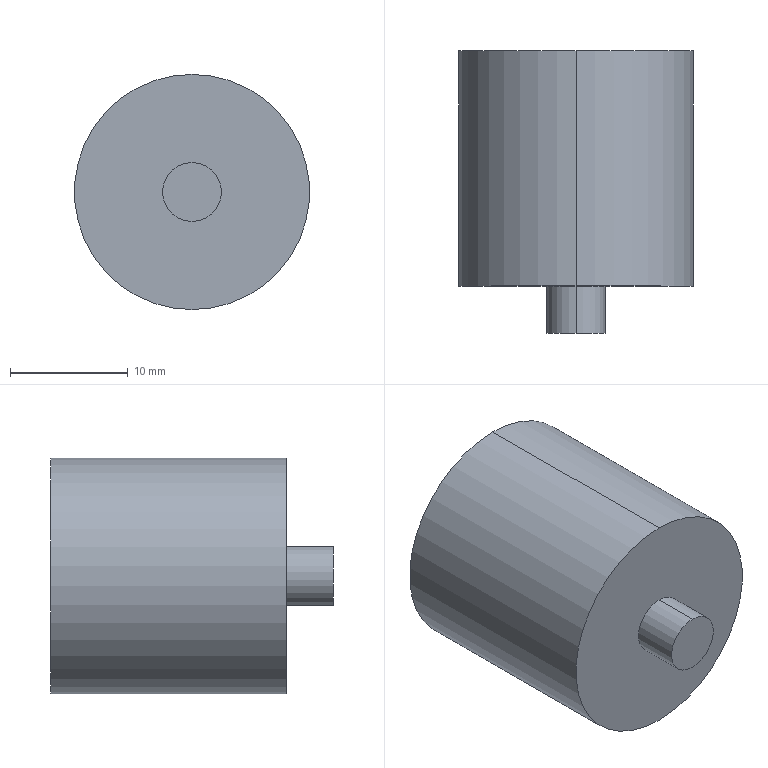Part | SolidWorks | features Revolution 1 | 1 solid | 7 faces | box 20 x 24 x 20 mm | volume 6362 mm3 | cylinder 4 | plane 3 | commonest cylinder face diameters 5 x2 20 x2
STEP:
#1=CARTESIAN_POINT('',(0.,0.4473,2.5));
#2=VERTEX_POINT('',#1);
#3=CARTESIAN_POINT('',(0.,0.4473,-2.5));
#4=VERTEX_POINT('',#3);
#5=CARTESIAN_POINT('',(0.,0.4473,0.));
#6=DIRECTION('',(0.,1.,0.));
#7=DIRECTION('',(0.,0.,1.));
#8=AXIS2_PLACEMENT_3D('',#5,#6,#7);
#9=CIRCLE('',#8,2.5);
#10=EDGE_CURVE('',#2,#4,#9,.T.);
#11=ORIENTED_EDGE('',*,*,#10,.T.);
#12=CARTESIAN_POINT('',(0.,4.447,-2.5));
#13=VERTEX_POINT('',#12);
#14=CARTESIAN_POINT('',(0.,8.623,-2.5));
#15=DIRECTION('',(0.,1.,0.));
#16=VECTOR('',#15,1000.);
#17=LINE('',#14,#16);
#18=EDGE_CURVE('',#4,#13,#17,.T.);
#19=ORIENTED_EDGE('',*,*,#18,.T.);
#20=CARTESIAN_POINT('',(0.,4.447,2.5));
#21=VERTEX_POINT('',#20);
#22=CARTESIAN_POINT('',(0.,4.447,0.));
#23=DIRECTION('',(0.,1.,0.));
#24=DIRECTION('',(0.,0.,1.));
#25=AXIS2_PLACEMENT_3D('',#22,#23,#24);
#26=CIRCLE('',#25,2.5);
#27=EDGE_CURVE('',#21,#13,#26,.T.);
#28=ORIENTED_EDGE('',*,*,#27,.F.);
#29=CARTESIAN_POINT('',(0.,8.623,2.5));
#30=DIRECTION('',(0.,1.,0.));
#31=VECTOR('',#30,1000.);
#32=LINE('',#29,#31);
#33=EDGE_CURVE('',#2,#21,#32,.T.);
#34=ORIENTED_EDGE('',*,*,#33,.F.);
#35=EDGE_LOOP('',(#11,#19,#28,#34));
#36=FACE_OUTER_BOUND('',#35,.T.);
#37=CARTESIAN_POINT('',(0.,8.623,0.));
#38=DIRECTION('',(0.,1.,0.));
#39=DIRECTION('',(0.,0.,1.));
#40=AXIS2_PLACEMENT_3D('',#37,#38,#39);
#41=CYLINDRICAL_SURFACE('',#40,2.5);
#42=ADVANCED_FACE('',(#36),#41,.T.);
#43=CARTESIAN_POINT('',(0.,4.447,10.));
#44=VERTEX_POINT('',#43);
#45=CARTESIAN_POINT('',(0.,4.447,-10.));
#46=VERTEX_POINT('',#45);
#47=CARTESIAN_POINT('',(0.,4.447,0.));
#48=DIRECTION('',(0.,1.,0.));
#49=DIRECTION('',(0.,0.,1.));
#50=AXIS2_PLACEMENT_3D('',#47,#48,#49);
#51=CIRCLE('',#50,10.);
#52=EDGE_CURVE('',#44,#46,#51,.T.);
#53=ORIENTED_EDGE('',*,*,#52,.T.);
#54=CARTESIAN_POINT('',(0.,24.447,-10.));
#55=VERTEX_POINT('',#54);
#56=CARTESIAN_POINT('',(0.,8.623,-10.));
#57=DIRECTION('',(0.,1.,0.));
#58=VECTOR('',#57,1000.);
#59=LINE('',#56,#58);
#60=EDGE_CURVE('',#46,#55,#59,.T.);
#61=ORIENTED_EDGE('',*,*,#60,.T.);
#62=CARTESIAN_POINT('',(0.,24.447,10.));
#63=VERTEX_POINT('',#62);
#64=CARTESIAN_POINT('',(0.,24.447,0.));
#65=DIRECTION('',(0.,1.,0.));
#66=DIRECTION('',(0.,0.,1.));
#67=AXIS2_PLACEMENT_3D('',#64,#65,#66);
#68=CIRCLE('',#67,10.);
#69=EDGE_CURVE('',#63,#55,#68,.T.);
#70=ORIENTED_EDGE('',*,*,#69,.F.);
#71=CARTESIAN_POINT('',(0.,8.623,10.));
#72=DIRECTION('',(0.,1.,0.));
#73=VECTOR('',#72,1000.);
#74=LINE('',#71,#73);
#75=EDGE_CURVE('',#44,#63,#74,.T.);
#76=ORIENTED_EDGE('',*,*,#75,.F.);
#77=EDGE_LOOP('',(#53,#61,#70,#76));
#78=FACE_OUTER_BOUND('',#77,.T.);
#79=CARTESIAN_POINT('',(0.,8.623,0.));
#80=DIRECTION('',(0.,1.,0.));
#81=DIRECTION('',(0.,0.,1.));
#82=AXIS2_PLACEMENT_3D('',#79,#80,#81);
#83=CYLINDRICAL_SURFACE('',#82,10.);
#84=ADVANCED_FACE('',(#78),#83,.T.);
#85=ORIENTED_EDGE('',*,*,#69,.T.);
#86=CARTESIAN_POINT('',(0.,24.447,0.));
#87=DIRECTION('',(0.,1.,0.));
#88=DIRECTION('',(0.,0.,1.));
#89=AXIS2_PLACEMENT_3D('',#86,#87,#88);
#90=CIRCLE('',#89,10.);
#91=EDGE_CURVE('',#55,#63,#90,.T.);
#92=ORIENTED_EDGE('',*,*,#91,.T.);
#93=EDGE_LOOP('',(#85,#92));
#94=FACE_OUTER_BOUND('',#93,.T.);
#95=CARTESIAN_POINT('',(0.,24.447,0.));
#96=DIRECTION('',(0.,-1.,0.));
#97=DIRECTION('',(0.,0.,-1.));
#98=AXIS2_PLACEMENT_3D('',#95,#96,#97);
#99=PLANE('',#98);
#100=ADVANCED_FACE('',(#94),#99,.F.);
#101=ORIENTED_EDGE('',*,*,#60,.F.);
#102=CARTESIAN_POINT('',(0.,4.447,0.));
#103=DIRECTION('',(0.,1.,0.));
#104=DIRECTION('',(0.,0.,1.));
#105=AXIS2_PLACEMENT_3D('',#102,#103,#104);
#106=CIRCLE('',#105,10.);
#107=EDGE_CURVE('',#46,#44,#106,.T.);
#108=ORIENTED_EDGE('',*,*,#107,.T.);
#109=ORIENTED_EDGE('',*,*,#75,.T.);
#110=ORIENTED_EDGE('',*,*,#91,.F.);
#111=EDGE_LOOP('',(#101,#108,#109,#110));
#112=FACE_OUTER_BOUND('',#111,.T.);
#113=CARTESIAN_POINT('',(0.,8.623,0.));
#114=DIRECTION('',(0.,1.,0.));
#115=DIRECTION('',(0.,0.,1.));
#116=AXIS2_PLACEMENT_3D('',#113,#114,#115);
#117=CYLINDRICAL_SURFACE('',#116,10.);
#118=ADVANCED_FACE('',(#112),#117,.T.);
#119=ORIENTED_EDGE('',*,*,#52,.F.);
#120=ORIENTED_EDGE('',*,*,#107,.F.);
#121=EDGE_LOOP('',(#119,#120));
#122=FACE_OUTER_BOUND('',#121,.T.);
#123=ORIENTED_EDGE('',*,*,#27,.T.);
#124=CARTESIAN_POINT('',(0.,4.447,0.));
#125=DIRECTION('',(0.,1.,0.));
#126=DIRECTION('',(0.,0.,1.));
#127=AXIS2_PLACEMENT_3D('',#124,#125,#126);
#128=CIRCLE('',#127,2.5);
#129=EDGE_CURVE('',#13,#21,#128,.T.);
#130=ORIENTED_EDGE('',*,*,#129,.T.);
#131=EDGE_LOOP('',(#123,#130));
#132=FACE_BOUND('',#131,.T.);
#133=CARTESIAN_POINT('',(10.,4.447,0.));
#134=DIRECTION('',(0.,1.,0.));
#135=DIRECTION('',(0.,0.,1.));
#136=AXIS2_PLACEMENT_3D('',#133,#134,#135);
#137=PLANE('',#136);
#138=ADVANCED_FACE('',(#122,#132),#137,.F.);
#139=ORIENTED_EDGE('',*,*,#18,.F.);
#140=CARTESIAN_POINT('',(0.,0.4473,0.));
#141=DIRECTION('',(0.,1.,0.));
#142=DIRECTION('',(0.,0.,1.));
#143=AXIS2_PLACEMENT_3D('',#140,#141,#142);
#144=CIRCLE('',#143,2.5);
#145=EDGE_CURVE('',#4,#2,#144,.T.);
#146=ORIENTED_EDGE('',*,*,#145,.T.);
#147=ORIENTED_EDGE('',*,*,#33,.T.);
#148=ORIENTED_EDGE('',*,*,#129,.F.);
#149=EDGE_LOOP('',(#139,#146,#147,#148));
#150=FACE_OUTER_BOUND('',#149,.T.);
#151=CARTESIAN_POINT('',(0.,8.623,0.));
#152=DIRECTION('',(0.,1.,0.));
#153=DIRECTION('',(0.,0.,1.));
#154=AXIS2_PLACEMENT_3D('',#151,#152,#153);
#155=CYLINDRICAL_SURFACE('',#154,2.5);
#156=ADVANCED_FACE('',(#150),#155,.T.);
#157=ORIENTED_EDGE('',*,*,#10,.F.);
#158=ORIENTED_EDGE('',*,*,#145,.F.);
#159=EDGE_LOOP('',(#157,#158));
#160=FACE_OUTER_BOUND('',#159,.T.);
#161=CARTESIAN_POINT('',(2.5,0.4473,0.));
#162=DIRECTION('',(0.,1.,0.));
#163=DIRECTION('',(0.,0.,1.));
#164=AXIS2_PLACEMENT_3D('',#161,#162,#163);
#165=PLANE('',#164);
#166=ADVANCED_FACE('',(#160),#165,.F.);
#167=CLOSED_SHELL('',(#42,#84,#100,#118,#138,#156,#166));
#168=MANIFOLD_SOLID_BREP('',#167);
#169=CARTESIAN_POINT('',(0.,0.,0.));
#170=DIRECTION('',(0.,0.,1.));
#171=DIRECTION('',(1.,0.,0.));
#172=AXIS2_PLACEMENT_3D('',#169,#170,#171);
#173=(LENGTH_UNIT()NAMED_UNIT(*)SI_UNIT(.MILLI.,.METRE.));
#174=UNCERTAINTY_MEASURE_WITH_UNIT(LENGTH_MEASURE(0.00001),#173,'','');
#175=(NAMED_UNIT(*)PLANE_ANGLE_UNIT()SI_UNIT($,.RADIAN.));
#176=(NAMED_UNIT(*)SI_UNIT($,.STERADIAN.)SOLID_ANGLE_UNIT());
#177=(GEOMETRIC_REPRESENTATION_CONTEXT(3)GLOBAL_UNCERTAINTY_ASSIGNED_CONTEXT((#174))GLOBAL_UNIT_ASSIGNED_CONTEXT((#173,#175,#176))REPRESENTATION_CONTEXT('',''));
#178=ADVANCED_BREP_SHAPE_REPRESENTATION('',(#168,#172),#177);